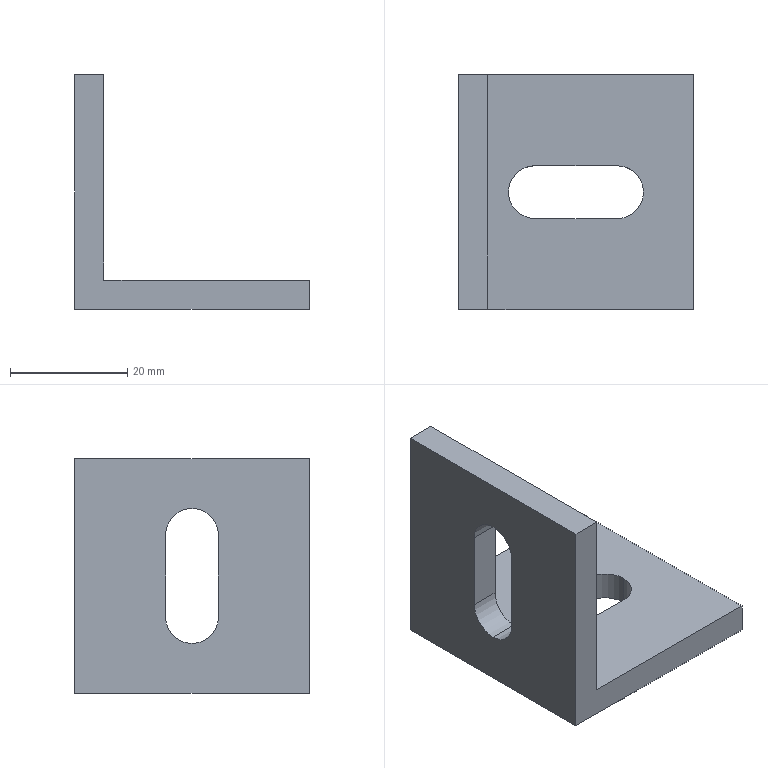Part | 1 solid | 18 faces | box 40 x 40 x 40 mm | volume 13104 mm3 | plane 12 | cylinder 6 | commonest cylinder face diameters 9 x6
STEP:
#1=CARTESIAN_POINT('',(0.,20.,8.5));
#2=VERTEX_POINT('',#1);
#3=CARTESIAN_POINT('',(0.,24.5,13.));
#4=VERTEX_POINT('',#3);
#5=CARTESIAN_POINT('',(0.,20.,13.));
#6=DIRECTION('',(1.,0.,0.));
#7=DIRECTION('',(0.,0.,-1.));
#8=AXIS2_PLACEMENT_3D('',#5,#6,#7);
#9=CIRCLE('',#8,4.5);
#10=EDGE_CURVE('',#2,#4,#9,.T.);
#11=ORIENTED_EDGE('',*,*,#10,.F.);
#12=CARTESIAN_POINT('',(5.,20.,8.5));
#13=VERTEX_POINT('',#12);
#14=CARTESIAN_POINT('',(0.,20.,8.5));
#15=DIRECTION('',(1.,0.,0.));
#16=VECTOR('',#15,1000.);
#17=LINE('',#14,#16);
#18=EDGE_CURVE('',#2,#13,#17,.T.);
#19=ORIENTED_EDGE('',*,*,#18,.T.);
#20=CARTESIAN_POINT('',(5.,24.5,13.));
#21=VERTEX_POINT('',#20);
#22=CARTESIAN_POINT('',(5.,20.,13.));
#23=DIRECTION('',(1.,0.,0.));
#24=DIRECTION('',(0.,0.,-1.));
#25=AXIS2_PLACEMENT_3D('',#22,#23,#24);
#26=CIRCLE('',#25,4.5);
#27=EDGE_CURVE('',#13,#21,#26,.T.);
#28=ORIENTED_EDGE('',*,*,#27,.T.);
#29=CARTESIAN_POINT('',(0.,24.5,13.));
#30=DIRECTION('',(1.,0.,0.));
#31=VECTOR('',#30,1000.);
#32=LINE('',#29,#31);
#33=EDGE_CURVE('',#4,#21,#32,.T.);
#34=ORIENTED_EDGE('',*,*,#33,.F.);
#35=EDGE_LOOP('',(#11,#19,#28,#34));
#36=FACE_OUTER_BOUND('',#35,.T.);
#37=CARTESIAN_POINT('',(0.,20.,13.));
#38=DIRECTION('',(1.,0.,0.));
#39=DIRECTION('',(0.,0.,-1.));
#40=AXIS2_PLACEMENT_3D('',#37,#38,#39);
#41=CYLINDRICAL_SURFACE('',#40,4.5);
#42=ADVANCED_FACE('',(#36),#41,.F.);
#43=CARTESIAN_POINT('',(31.5,20.,0.));
#44=VERTEX_POINT('',#43);
#45=CARTESIAN_POINT('',(27.,24.5,0.));
#46=VERTEX_POINT('',#45);
#47=CARTESIAN_POINT('',(27.,20.,0.));
#48=DIRECTION('',(0.,0.,1.));
#49=DIRECTION('',(1.,0.,0.));
#50=AXIS2_PLACEMENT_3D('',#47,#48,#49);
#51=CIRCLE('',#50,4.5);
#52=EDGE_CURVE('',#44,#46,#51,.T.);
#53=ORIENTED_EDGE('',*,*,#52,.F.);
#54=CARTESIAN_POINT('',(31.5,20.,5.));
#55=VERTEX_POINT('',#54);
#56=CARTESIAN_POINT('',(31.5,20.,0.));
#57=DIRECTION('',(0.,0.,1.));
#58=VECTOR('',#57,1000.);
#59=LINE('',#56,#58);
#60=EDGE_CURVE('',#44,#55,#59,.T.);
#61=ORIENTED_EDGE('',*,*,#60,.T.);
#62=CARTESIAN_POINT('',(27.,24.5,5.));
#63=VERTEX_POINT('',#62);
#64=CARTESIAN_POINT('',(27.,20.,5.));
#65=DIRECTION('',(0.,0.,1.));
#66=DIRECTION('',(1.,0.,0.));
#67=AXIS2_PLACEMENT_3D('',#64,#65,#66);
#68=CIRCLE('',#67,4.5);
#69=EDGE_CURVE('',#55,#63,#68,.T.);
#70=ORIENTED_EDGE('',*,*,#69,.T.);
#71=CARTESIAN_POINT('',(27.,24.5,0.));
#72=DIRECTION('',(0.,0.,1.));
#73=VECTOR('',#72,1000.);
#74=LINE('',#71,#73);
#75=EDGE_CURVE('',#46,#63,#74,.T.);
#76=ORIENTED_EDGE('',*,*,#75,.F.);
#77=EDGE_LOOP('',(#53,#61,#70,#76));
#78=FACE_OUTER_BOUND('',#77,.T.);
#79=CARTESIAN_POINT('',(27.,20.,0.));
#80=DIRECTION('',(0.,0.,1.));
#81=DIRECTION('',(1.,0.,0.));
#82=AXIS2_PLACEMENT_3D('',#79,#80,#81);
#83=CYLINDRICAL_SURFACE('',#82,4.5);
#84=ADVANCED_FACE('',(#78),#83,.F.);
#85=CARTESIAN_POINT('',(5.,40.,5.));
#86=VERTEX_POINT('',#85);
#87=CARTESIAN_POINT('',(5.,40.,40.));
#88=VERTEX_POINT('',#87);
#89=CARTESIAN_POINT('',(5.,40.,5.));
#90=DIRECTION('',(0.,0.,1.));
#91=VECTOR('',#90,1000.);
#92=LINE('',#89,#91);
#93=EDGE_CURVE('',#86,#88,#92,.T.);
#94=ORIENTED_EDGE('',*,*,#93,.F.);
#95=CARTESIAN_POINT('',(40.,40.,5.));
#96=VERTEX_POINT('',#95);
#97=CARTESIAN_POINT('',(40.,40.,5.));
#98=DIRECTION('',(-1.,0.,0.));
#99=VECTOR('',#98,1000.);
#100=LINE('',#97,#99);
#101=EDGE_CURVE('',#96,#86,#100,.T.);
#102=ORIENTED_EDGE('',*,*,#101,.F.);
#103=CARTESIAN_POINT('',(40.,40.,0.));
#104=VERTEX_POINT('',#103);
#105=CARTESIAN_POINT('',(40.,40.,40.));
#106=DIRECTION('',(0.,0.,-1.));
#107=VECTOR('',#106,1000.);
#108=LINE('',#105,#107);
#109=EDGE_CURVE('',#96,#104,#108,.T.);
#110=ORIENTED_EDGE('',*,*,#109,.T.);
#111=CARTESIAN_POINT('',(0.,40.,0.));
#112=VERTEX_POINT('',#111);
#113=CARTESIAN_POINT('',(40.,40.,0.));
#114=DIRECTION('',(-1.,0.,0.));
#115=VECTOR('',#114,1000.);
#116=LINE('',#113,#115);
#117=EDGE_CURVE('',#104,#112,#116,.T.);
#118=ORIENTED_EDGE('',*,*,#117,.T.);
#119=CARTESIAN_POINT('',(0.,40.,40.));
#120=VERTEX_POINT('',#119);
#121=CARTESIAN_POINT('',(0.,40.,40.));
#122=DIRECTION('',(0.,0.,-1.));
#123=VECTOR('',#122,1000.);
#124=LINE('',#121,#123);
#125=EDGE_CURVE('',#120,#112,#124,.T.);
#126=ORIENTED_EDGE('',*,*,#125,.F.);
#127=CARTESIAN_POINT('',(40.,40.,40.));
#128=DIRECTION('',(-1.,0.,0.));
#129=VECTOR('',#128,1000.);
#130=LINE('',#127,#129);
#131=EDGE_CURVE('',#88,#120,#130,.T.);
#132=ORIENTED_EDGE('',*,*,#131,.F.);
#133=EDGE_LOOP('',(#94,#102,#110,#118,#126,#132));
#134=FACE_OUTER_BOUND('',#133,.T.);
#135=CARTESIAN_POINT('',(40.,40.,40.));
#136=DIRECTION('',(0.,1.,0.));
#137=DIRECTION('',(0.,0.,1.));
#138=AXIS2_PLACEMENT_3D('',#135,#136,#137);
#139=PLANE('',#138);
#140=ADVANCED_FACE('',(#134),#139,.T.);
#141=CARTESIAN_POINT('',(5.,0.,40.));
#142=VERTEX_POINT('',#141);
#143=CARTESIAN_POINT('',(5.,0.,40.));
#144=DIRECTION('',(0.,1.,0.));
#145=VECTOR('',#144,1000.);
#146=LINE('',#143,#145);
#147=EDGE_CURVE('',#142,#88,#146,.T.);
#148=ORIENTED_EDGE('',*,*,#147,.T.);
#149=ORIENTED_EDGE('',*,*,#131,.T.);
#150=CARTESIAN_POINT('',(0.,0.,40.));
#151=VERTEX_POINT('',#150);
#152=CARTESIAN_POINT('',(0.,0.,40.));
#153=DIRECTION('',(0.,1.,0.));
#154=VECTOR('',#153,1000.);
#155=LINE('',#152,#154);
#156=EDGE_CURVE('',#151,#120,#155,.T.);
#157=ORIENTED_EDGE('',*,*,#156,.F.);
#158=CARTESIAN_POINT('',(40.,0.,40.));
#159=DIRECTION('',(-1.,0.,0.));
#160=VECTOR('',#159,1000.);
#161=LINE('',#158,#160);
#162=EDGE_CURVE('',#142,#151,#161,.T.);
#163=ORIENTED_EDGE('',*,*,#162,.F.);
#164=EDGE_LOOP('',(#148,#149,#157,#163));
#165=FACE_OUTER_BOUND('',#164,.T.);
#166=CARTESIAN_POINT('',(40.,0.,40.));
#167=DIRECTION('',(0.,0.,1.));
#168=DIRECTION('',(1.,0.,0.));
#169=AXIS2_PLACEMENT_3D('',#166,#167,#168);
#170=PLANE('',#169);
#171=ADVANCED_FACE('',(#165),#170,.T.);
#172=CARTESIAN_POINT('',(5.,0.,5.));
#173=VERTEX_POINT('',#172);
#174=CARTESIAN_POINT('',(5.,0.,5.));
#175=DIRECTION('',(0.,0.,1.));
#176=VECTOR('',#175,1000.);
#177=LINE('',#174,#176);
#178=EDGE_CURVE('',#173,#142,#177,.T.);
#179=ORIENTED_EDGE('',*,*,#178,.T.);
#180=ORIENTED_EDGE('',*,*,#162,.T.);
#181=CARTESIAN_POINT('',(0.,0.,0.));
#182=VERTEX_POINT('',#181);
#183=CARTESIAN_POINT('',(0.,0.,0.));
#184=DIRECTION('',(0.,0.,1.));
#185=VECTOR('',#184,1000.);
#186=LINE('',#183,#185);
#187=EDGE_CURVE('',#182,#151,#186,.T.);
#188=ORIENTED_EDGE('',*,*,#187,.F.);
#189=CARTESIAN_POINT('',(40.,0.,0.));
#190=VERTEX_POINT('',#189);
#191=CARTESIAN_POINT('',(40.,0.,0.));
#192=DIRECTION('',(-1.,0.,0.));
#193=VECTOR('',#192,1000.);
#194=LINE('',#191,#193);
#195=EDGE_CURVE('',#190,#182,#194,.T.);
#196=ORIENTED_EDGE('',*,*,#195,.F.);
#197=CARTESIAN_POINT('',(40.,0.,5.));
#198=VERTEX_POINT('',#197);
#199=CARTESIAN_POINT('',(40.,0.,0.));
#200=DIRECTION('',(0.,0.,1.));
#201=VECTOR('',#200,1000.);
#202=LINE('',#199,#201);
#203=EDGE_CURVE('',#190,#198,#202,.T.);
#204=ORIENTED_EDGE('',*,*,#203,.T.);
#205=CARTESIAN_POINT('',(40.,0.,5.));
#206=DIRECTION('',(-1.,0.,0.));
#207=VECTOR('',#206,1000.);
#208=LINE('',#205,#207);
#209=EDGE_CURVE('',#198,#173,#208,.T.);
#210=ORIENTED_EDGE('',*,*,#209,.T.);
#211=EDGE_LOOP('',(#179,#180,#188,#196,#204,#210));
#212=FACE_OUTER_BOUND('',#211,.T.);
#213=CARTESIAN_POINT('',(40.,0.,0.));
#214=DIRECTION('',(0.,-1.,0.));
#215=DIRECTION('',(0.,0.,-1.));
#216=AXIS2_PLACEMENT_3D('',#213,#214,#215);
#217=PLANE('',#216);
#218=ADVANCED_FACE('',(#212),#217,.T.);
#219=CARTESIAN_POINT('',(27.,15.5,0.));
#220=VERTEX_POINT('',#219);
#221=CARTESIAN_POINT('',(27.,20.,0.));
#222=DIRECTION('',(0.,0.,1.));
#223=DIRECTION('',(1.,0.,0.));
#224=AXIS2_PLACEMENT_3D('',#221,#222,#223);
#225=CIRCLE('',#224,4.5);
#226=EDGE_CURVE('',#220,#44,#225,.T.);
#227=ORIENTED_EDGE('',*,*,#226,.T.);
#228=ORIENTED_EDGE('',*,*,#52,.T.);
#229=CARTESIAN_POINT('',(13.,24.5,0.));
#230=VERTEX_POINT('',#229);
#231=CARTESIAN_POINT('',(27.,24.5,0.));
#232=DIRECTION('',(-1.,0.,0.));
#233=VECTOR('',#232,1000.);
#234=LINE('',#231,#233);
#235=EDGE_CURVE('',#46,#230,#234,.T.);
#236=ORIENTED_EDGE('',*,*,#235,.T.);
#237=CARTESIAN_POINT('',(13.,15.5,0.));
#238=VERTEX_POINT('',#237);
#239=CARTESIAN_POINT('',(13.,20.,0.));
#240=DIRECTION('',(0.,0.,1.));
#241=DIRECTION('',(1.,0.,0.));
#242=AXIS2_PLACEMENT_3D('',#239,#240,#241);
#243=CIRCLE('',#242,4.5);
#244=EDGE_CURVE('',#230,#238,#243,.T.);
#245=ORIENTED_EDGE('',*,*,#244,.T.);
#246=CARTESIAN_POINT('',(13.,15.5,0.));
#247=DIRECTION('',(1.,0.,0.));
#248=VECTOR('',#247,1000.);
#249=LINE('',#246,#248);
#250=EDGE_CURVE('',#238,#220,#249,.T.);
#251=ORIENTED_EDGE('',*,*,#250,.T.);
#252=EDGE_LOOP('',(#227,#228,#236,#245,#251));
#253=FACE_BOUND('',#252,.T.);
#254=CARTESIAN_POINT('',(0.,40.,0.));
#255=DIRECTION('',(0.,-1.,0.));
#256=VECTOR('',#255,1000.);
#257=LINE('',#254,#256);
#258=EDGE_CURVE('',#112,#182,#257,.T.);
#259=ORIENTED_EDGE('',*,*,#258,.F.);
#260=ORIENTED_EDGE('',*,*,#117,.F.);
#261=CARTESIAN_POINT('',(40.,40.,0.));
#262=DIRECTION('',(0.,-1.,0.));
#263=VECTOR('',#262,1000.);
#264=LINE('',#261,#263);
#265=EDGE_CURVE('',#104,#190,#264,.T.);
#266=ORIENTED_EDGE('',*,*,#265,.T.);
#267=ORIENTED_EDGE('',*,*,#195,.T.);
#268=EDGE_LOOP('',(#259,#260,#266,#267));
#269=FACE_OUTER_BOUND('',#268,.T.);
#270=CARTESIAN_POINT('',(40.,40.,0.));
#271=DIRECTION('',(0.,0.,-1.));
#272=DIRECTION('',(-1.,0.,0.));
#273=AXIS2_PLACEMENT_3D('',#270,#271,#272);
#274=PLANE('',#273);
#275=ADVANCED_FACE('',(#253,#269),#274,.T.);
#276=ORIENTED_EDGE('',*,*,#109,.F.);
#277=CARTESIAN_POINT('',(40.,0.,5.));
#278=DIRECTION('',(0.,1.,0.));
#279=VECTOR('',#278,1000.);
#280=LINE('',#277,#279);
#281=EDGE_CURVE('',#198,#96,#280,.T.);
#282=ORIENTED_EDGE('',*,*,#281,.F.);
#283=ORIENTED_EDGE('',*,*,#203,.F.);
#284=ORIENTED_EDGE('',*,*,#265,.F.);
#285=EDGE_LOOP('',(#276,#282,#283,#284));
#286=FACE_OUTER_BOUND('',#285,.T.);
#287=CARTESIAN_POINT('',(40.,0.,0.));
#288=DIRECTION('',(-1.,0.,0.));
#289=DIRECTION('',(0.,0.,1.));
#290=AXIS2_PLACEMENT_3D('',#287,#288,#289);
#291=PLANE('',#290);
#292=ADVANCED_FACE('',(#286),#291,.F.);
#293=CARTESIAN_POINT('',(0.,24.5,27.));
#294=VERTEX_POINT('',#293);
#295=CARTESIAN_POINT('',(0.,15.5,27.));
#296=VERTEX_POINT('',#295);
#297=CARTESIAN_POINT('',(0.,20.,27.));
#298=DIRECTION('',(1.,0.,0.));
#299=DIRECTION('',(0.,0.,-1.));
#300=AXIS2_PLACEMENT_3D('',#297,#298,#299);
#301=CIRCLE('',#300,4.5);
#302=EDGE_CURVE('',#294,#296,#301,.T.);
#303=ORIENTED_EDGE('',*,*,#302,.T.);
#304=CARTESIAN_POINT('',(0.,15.5,13.));
#305=VERTEX_POINT('',#304);
#306=CARTESIAN_POINT('',(0.,15.5,27.));
#307=DIRECTION('',(0.,0.,-1.));
#308=VECTOR('',#307,1000.);
#309=LINE('',#306,#308);
#310=EDGE_CURVE('',#296,#305,#309,.T.);
#311=ORIENTED_EDGE('',*,*,#310,.T.);
#312=CARTESIAN_POINT('',(0.,20.,13.));
#313=DIRECTION('',(1.,0.,0.));
#314=DIRECTION('',(0.,0.,-1.));
#315=AXIS2_PLACEMENT_3D('',#312,#313,#314);
#316=CIRCLE('',#315,4.5);
#317=EDGE_CURVE('',#305,#2,#316,.T.);
#318=ORIENTED_EDGE('',*,*,#317,.T.);
#319=ORIENTED_EDGE('',*,*,#10,.T.);
#320=CARTESIAN_POINT('',(0.,24.5,13.));
#321=DIRECTION('',(0.,0.,1.));
#322=VECTOR('',#321,1000.);
#323=LINE('',#320,#322);
#324=EDGE_CURVE('',#4,#294,#323,.T.);
#325=ORIENTED_EDGE('',*,*,#324,.T.);
#326=EDGE_LOOP('',(#303,#311,#318,#319,#325));
#327=FACE_BOUND('',#326,.T.);
#328=ORIENTED_EDGE('',*,*,#125,.T.);
#329=ORIENTED_EDGE('',*,*,#258,.T.);
#330=ORIENTED_EDGE('',*,*,#187,.T.);
#331=ORIENTED_EDGE('',*,*,#156,.T.);
#332=EDGE_LOOP('',(#328,#329,#330,#331));
#333=FACE_OUTER_BOUND('',#332,.T.);
#334=CARTESIAN_POINT('',(0.,0.,0.));
#335=DIRECTION('',(-1.,0.,0.));
#336=DIRECTION('',(0.,0.,1.));
#337=AXIS2_PLACEMENT_3D('',#334,#335,#336);
#338=PLANE('',#337);
#339=ADVANCED_FACE('',(#327,#333),#338,.T.);
#340=CARTESIAN_POINT('',(5.,15.5,27.));
#341=VERTEX_POINT('',#340);
#342=CARTESIAN_POINT('',(5.,15.5,13.));
#343=VERTEX_POINT('',#342);
#344=CARTESIAN_POINT('',(5.,15.5,27.));
#345=DIRECTION('',(0.,0.,-1.));
#346=VECTOR('',#345,1000.);
#347=LINE('',#344,#346);
#348=EDGE_CURVE('',#341,#343,#347,.T.);
#349=ORIENTED_EDGE('',*,*,#348,.F.);
#350=CARTESIAN_POINT('',(5.,24.5,27.));
#351=VERTEX_POINT('',#350);
#352=CARTESIAN_POINT('',(5.,20.,27.));
#353=DIRECTION('',(1.,0.,0.));
#354=DIRECTION('',(0.,0.,-1.));
#355=AXIS2_PLACEMENT_3D('',#352,#353,#354);
#356=CIRCLE('',#355,4.5);
#357=EDGE_CURVE('',#351,#341,#356,.T.);
#358=ORIENTED_EDGE('',*,*,#357,.F.);
#359=CARTESIAN_POINT('',(5.,24.5,13.));
#360=DIRECTION('',(0.,0.,1.));
#361=VECTOR('',#360,1000.);
#362=LINE('',#359,#361);
#363=EDGE_CURVE('',#21,#351,#362,.T.);
#364=ORIENTED_EDGE('',*,*,#363,.F.);
#365=ORIENTED_EDGE('',*,*,#27,.F.);
#366=CARTESIAN_POINT('',(5.,20.,13.));
#367=DIRECTION('',(1.,0.,0.));
#368=DIRECTION('',(0.,0.,-1.));
#369=AXIS2_PLACEMENT_3D('',#366,#367,#368);
#370=CIRCLE('',#369,4.5);
#371=EDGE_CURVE('',#343,#13,#370,.T.);
#372=ORIENTED_EDGE('',*,*,#371,.F.);
#373=EDGE_LOOP('',(#349,#358,#364,#365,#372));
#374=FACE_BOUND('',#373,.T.);
#375=ORIENTED_EDGE('',*,*,#93,.T.);
#376=ORIENTED_EDGE('',*,*,#147,.F.);
#377=ORIENTED_EDGE('',*,*,#178,.F.);
#378=CARTESIAN_POINT('',(5.,0.,5.));
#379=DIRECTION('',(0.,1.,0.));
#380=VECTOR('',#379,1000.);
#381=LINE('',#378,#380);
#382=EDGE_CURVE('',#173,#86,#381,.T.);
#383=ORIENTED_EDGE('',*,*,#382,.T.);
#384=EDGE_LOOP('',(#375,#376,#377,#383));
#385=FACE_OUTER_BOUND('',#384,.T.);
#386=CARTESIAN_POINT('',(5.,0.,5.));
#387=DIRECTION('',(-1.,0.,0.));
#388=DIRECTION('',(0.,0.,1.));
#389=AXIS2_PLACEMENT_3D('',#386,#387,#388);
#390=PLANE('',#389);
#391=ADVANCED_FACE('',(#374,#385),#390,.F.);
#392=CARTESIAN_POINT('',(13.,24.5,5.));
#393=VERTEX_POINT('',#392);
#394=CARTESIAN_POINT('',(27.,24.5,5.));
#395=DIRECTION('',(-1.,0.,0.));
#396=VECTOR('',#395,1000.);
#397=LINE('',#394,#396);
#398=EDGE_CURVE('',#63,#393,#397,.T.);
#399=ORIENTED_EDGE('',*,*,#398,.F.);
#400=ORIENTED_EDGE('',*,*,#69,.F.);
#401=CARTESIAN_POINT('',(27.,15.5,5.));
#402=VERTEX_POINT('',#401);
#403=CARTESIAN_POINT('',(27.,20.,5.));
#404=DIRECTION('',(0.,0.,1.));
#405=DIRECTION('',(1.,0.,0.));
#406=AXIS2_PLACEMENT_3D('',#403,#404,#405);
#407=CIRCLE('',#406,4.5);
#408=EDGE_CURVE('',#402,#55,#407,.T.);
#409=ORIENTED_EDGE('',*,*,#408,.F.);
#410=CARTESIAN_POINT('',(13.,15.5,5.));
#411=VERTEX_POINT('',#410);
#412=CARTESIAN_POINT('',(13.,15.5,5.));
#413=DIRECTION('',(1.,0.,0.));
#414=VECTOR('',#413,1000.);
#415=LINE('',#412,#414);
#416=EDGE_CURVE('',#411,#402,#415,.T.);
#417=ORIENTED_EDGE('',*,*,#416,.F.);
#418=CARTESIAN_POINT('',(13.,20.,5.));
#419=DIRECTION('',(0.,0.,1.));
#420=DIRECTION('',(1.,0.,0.));
#421=AXIS2_PLACEMENT_3D('',#418,#419,#420);
#422=CIRCLE('',#421,4.5);
#423=EDGE_CURVE('',#393,#411,#422,.T.);
#424=ORIENTED_EDGE('',*,*,#423,.F.);
#425=EDGE_LOOP('',(#399,#400,#409,#417,#424));
#426=FACE_BOUND('',#425,.T.);
#427=ORIENTED_EDGE('',*,*,#101,.T.);
#428=ORIENTED_EDGE('',*,*,#382,.F.);
#429=ORIENTED_EDGE('',*,*,#209,.F.);
#430=ORIENTED_EDGE('',*,*,#281,.T.);
#431=EDGE_LOOP('',(#427,#428,#429,#430));
#432=FACE_OUTER_BOUND('',#431,.T.);
#433=CARTESIAN_POINT('',(40.,0.,5.));
#434=DIRECTION('',(0.,0.,-1.));
#435=DIRECTION('',(-1.,0.,0.));
#436=AXIS2_PLACEMENT_3D('',#433,#434,#435);
#437=PLANE('',#436);
#438=ADVANCED_FACE('',(#426,#432),#437,.F.);
#439=ORIENTED_EDGE('',*,*,#60,.F.);
#440=ORIENTED_EDGE('',*,*,#226,.F.);
#441=CARTESIAN_POINT('',(27.,15.5,0.));
#442=DIRECTION('',(0.,0.,1.));
#443=VECTOR('',#442,1000.);
#444=LINE('',#441,#443);
#445=EDGE_CURVE('',#220,#402,#444,.T.);
#446=ORIENTED_EDGE('',*,*,#445,.T.);
#447=ORIENTED_EDGE('',*,*,#408,.T.);
#448=EDGE_LOOP('',(#439,#440,#446,#447));
#449=FACE_OUTER_BOUND('',#448,.T.);
#450=CARTESIAN_POINT('',(27.,20.,0.));
#451=DIRECTION('',(0.,0.,1.));
#452=DIRECTION('',(1.,0.,0.));
#453=AXIS2_PLACEMENT_3D('',#450,#451,#452);
#454=CYLINDRICAL_SURFACE('',#453,4.5);
#455=ADVANCED_FACE('',(#449),#454,.F.);
#456=ORIENTED_EDGE('',*,*,#416,.T.);
#457=ORIENTED_EDGE('',*,*,#445,.F.);
#458=ORIENTED_EDGE('',*,*,#250,.F.);
#459=CARTESIAN_POINT('',(13.,15.5,0.));
#460=DIRECTION('',(0.,0.,1.));
#461=VECTOR('',#460,1000.);
#462=LINE('',#459,#461);
#463=EDGE_CURVE('',#238,#411,#462,.T.);
#464=ORIENTED_EDGE('',*,*,#463,.T.);
#465=EDGE_LOOP('',(#456,#457,#458,#464));
#466=FACE_OUTER_BOUND('',#465,.T.);
#467=CARTESIAN_POINT('',(13.,15.5,0.));
#468=DIRECTION('',(0.,-1.,0.));
#469=DIRECTION('',(0.,0.,-1.));
#470=AXIS2_PLACEMENT_3D('',#467,#468,#469);
#471=PLANE('',#470);
#472=ADVANCED_FACE('',(#466),#471,.F.);
#473=ORIENTED_EDGE('',*,*,#423,.T.);
#474=ORIENTED_EDGE('',*,*,#463,.F.);
#475=ORIENTED_EDGE('',*,*,#244,.F.);
#476=CARTESIAN_POINT('',(13.,24.5,0.));
#477=DIRECTION('',(0.,0.,1.));
#478=VECTOR('',#477,1000.);
#479=LINE('',#476,#478);
#480=EDGE_CURVE('',#230,#393,#479,.T.);
#481=ORIENTED_EDGE('',*,*,#480,.T.);
#482=EDGE_LOOP('',(#473,#474,#475,#481));
#483=FACE_OUTER_BOUND('',#482,.T.);
#484=CARTESIAN_POINT('',(13.,20.,0.));
#485=DIRECTION('',(0.,0.,1.));
#486=DIRECTION('',(1.,0.,0.));
#487=AXIS2_PLACEMENT_3D('',#484,#485,#486);
#488=CYLINDRICAL_SURFACE('',#487,4.5);
#489=ADVANCED_FACE('',(#483),#488,.F.);
#490=ORIENTED_EDGE('',*,*,#398,.T.);
#491=ORIENTED_EDGE('',*,*,#480,.F.);
#492=ORIENTED_EDGE('',*,*,#235,.F.);
#493=ORIENTED_EDGE('',*,*,#75,.T.);
#494=EDGE_LOOP('',(#490,#491,#492,#493));
#495=FACE_OUTER_BOUND('',#494,.T.);
#496=CARTESIAN_POINT('',(27.,24.5,0.));
#497=DIRECTION('',(0.,1.,0.));
#498=DIRECTION('',(0.,0.,1.));
#499=AXIS2_PLACEMENT_3D('',#496,#497,#498);
#500=PLANE('',#499);
#501=ADVANCED_FACE('',(#495),#500,.F.);
#502=ORIENTED_EDGE('',*,*,#357,.T.);
#503=CARTESIAN_POINT('',(0.,15.5,27.));
#504=DIRECTION('',(1.,0.,0.));
#505=VECTOR('',#504,1000.);
#506=LINE('',#503,#505);
#507=EDGE_CURVE('',#296,#341,#506,.T.);
#508=ORIENTED_EDGE('',*,*,#507,.F.);
#509=ORIENTED_EDGE('',*,*,#302,.F.);
#510=CARTESIAN_POINT('',(0.,24.5,27.));
#511=DIRECTION('',(1.,0.,0.));
#512=VECTOR('',#511,1000.);
#513=LINE('',#510,#512);
#514=EDGE_CURVE('',#294,#351,#513,.T.);
#515=ORIENTED_EDGE('',*,*,#514,.T.);
#516=EDGE_LOOP('',(#502,#508,#509,#515));
#517=FACE_OUTER_BOUND('',#516,.T.);
#518=CARTESIAN_POINT('',(0.,20.,27.));
#519=DIRECTION('',(1.,0.,0.));
#520=DIRECTION('',(0.,0.,-1.));
#521=AXIS2_PLACEMENT_3D('',#518,#519,#520);
#522=CYLINDRICAL_SURFACE('',#521,4.5);
#523=ADVANCED_FACE('',(#517),#522,.F.);
#524=ORIENTED_EDGE('',*,*,#363,.T.);
#525=ORIENTED_EDGE('',*,*,#514,.F.);
#526=ORIENTED_EDGE('',*,*,#324,.F.);
#527=ORIENTED_EDGE('',*,*,#33,.T.);
#528=EDGE_LOOP('',(#524,#525,#526,#527));
#529=FACE_OUTER_BOUND('',#528,.T.);
#530=CARTESIAN_POINT('',(0.,24.5,13.));
#531=DIRECTION('',(0.,1.,0.));
#532=DIRECTION('',(0.,0.,1.));
#533=AXIS2_PLACEMENT_3D('',#530,#531,#532);
#534=PLANE('',#533);
#535=ADVANCED_FACE('',(#529),#534,.F.);
#536=ORIENTED_EDGE('',*,*,#18,.F.);
#537=ORIENTED_EDGE('',*,*,#317,.F.);
#538=CARTESIAN_POINT('',(0.,15.5,13.));
#539=DIRECTION('',(1.,0.,0.));
#540=VECTOR('',#539,1000.);
#541=LINE('',#538,#540);
#542=EDGE_CURVE('',#305,#343,#541,.T.);
#543=ORIENTED_EDGE('',*,*,#542,.T.);
#544=ORIENTED_EDGE('',*,*,#371,.T.);
#545=EDGE_LOOP('',(#536,#537,#543,#544));
#546=FACE_OUTER_BOUND('',#545,.T.);
#547=CARTESIAN_POINT('',(0.,20.,13.));
#548=DIRECTION('',(1.,0.,0.));
#549=DIRECTION('',(0.,0.,-1.));
#550=AXIS2_PLACEMENT_3D('',#547,#548,#549);
#551=CYLINDRICAL_SURFACE('',#550,4.5);
#552=ADVANCED_FACE('',(#546),#551,.F.);
#553=ORIENTED_EDGE('',*,*,#348,.T.);
#554=ORIENTED_EDGE('',*,*,#542,.F.);
#555=ORIENTED_EDGE('',*,*,#310,.F.);
#556=ORIENTED_EDGE('',*,*,#507,.T.);
#557=EDGE_LOOP('',(#553,#554,#555,#556));
#558=FACE_OUTER_BOUND('',#557,.T.);
#559=CARTESIAN_POINT('',(0.,15.5,27.));
#560=DIRECTION('',(0.,-1.,0.));
#561=DIRECTION('',(0.,0.,-1.));
#562=AXIS2_PLACEMENT_3D('',#559,#560,#561);
#563=PLANE('',#562);
#564=ADVANCED_FACE('',(#558),#563,.F.);
#565=CLOSED_SHELL('',(#42,#84,#140,#171,#218,#275,#292,#339,#391,#438,#455,#472,#489,#501,#523,#535,#552,#564));
#566=MANIFOLD_SOLID_BREP('',#565);
#567=CARTESIAN_POINT('',(0.,0.,0.));
#568=DIRECTION('',(0.,0.,1.));
#569=DIRECTION('',(1.,0.,0.));
#570=AXIS2_PLACEMENT_3D('',#567,#568,#569);
#571=(LENGTH_UNIT()NAMED_UNIT(*)SI_UNIT(.MILLI.,.METRE.));
#572=UNCERTAINTY_MEASURE_WITH_UNIT(LENGTH_MEASURE(0.00001),#571,'','');
#573=(NAMED_UNIT(*)PLANE_ANGLE_UNIT()SI_UNIT($,.RADIAN.));
#574=(NAMED_UNIT(*)SI_UNIT($,.STERADIAN.)SOLID_ANGLE_UNIT());
#575=(GEOMETRIC_REPRESENTATION_CONTEXT(3)GLOBAL_UNCERTAINTY_ASSIGNED_CONTEXT((#572))GLOBAL_UNIT_ASSIGNED_CONTEXT((#571,#573,#574))REPRESENTATION_CONTEXT('',''));
#576=ADVANCED_BREP_SHAPE_REPRESENTATION('',(#566,#570),#575);